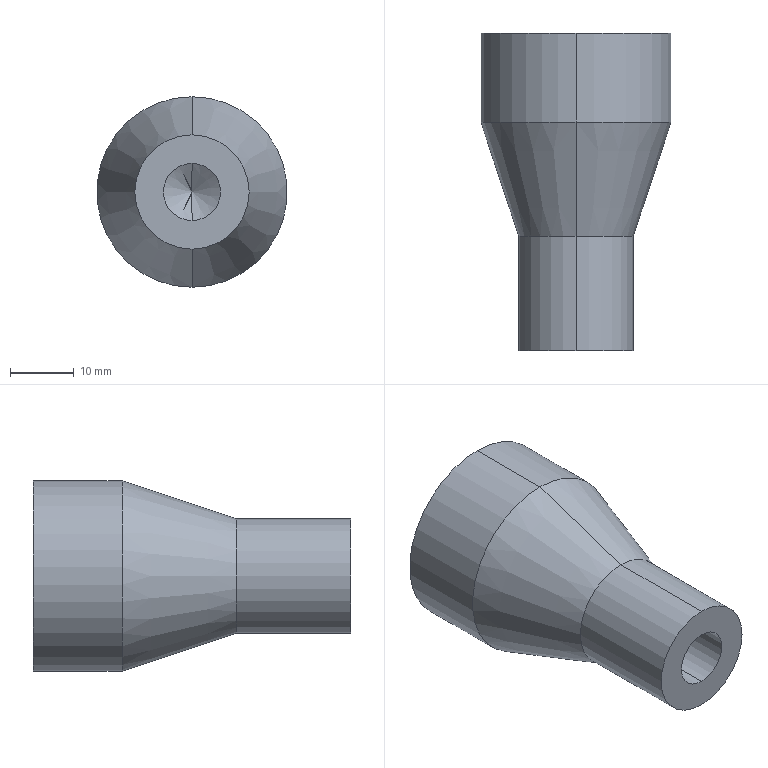Part | SolidWorks | features HoleWzd 2, Revolution 1 | 1 solid | 19 faces | box 30 x 50 x 30 mm | volume 17999 mm3 | cylinder 10 | cone 6 | plane 3 | commonest cylinder face diameters 3.3 x2 9 x2 18 x2 27 x2 30 x2
STEP:
#1=CARTESIAN_POINT('',(0.,34.9,-1.65));
#2=VERTEX_POINT('',#1);
#3=CARTESIAN_POINT('',(0.,34.9,1.65));
#4=VERTEX_POINT('',#3);
#5=CARTESIAN_POINT('',(0.,34.9,0.));
#6=DIRECTION('',(0.,1.,0.));
#7=DIRECTION('',(0.,0.,1.));
#8=AXIS2_PLACEMENT_3D('',#5,#6,#7);
#9=CIRCLE('',#8,1.65);
#10=EDGE_CURVE('',#2,#4,#9,.T.);
#11=ORIENTED_EDGE('',*,*,#10,.F.);
#12=CARTESIAN_POINT('',(0.,45.,-1.65));
#13=VERTEX_POINT('',#12);
#14=CARTESIAN_POINT('',(0.,45.,-1.65));
#15=DIRECTION('',(0.,1.,0.));
#16=VECTOR('',#15,1000.);
#17=LINE('',#14,#16);
#18=EDGE_CURVE('',#2,#13,#17,.T.);
#19=ORIENTED_EDGE('',*,*,#18,.T.);
#20=CARTESIAN_POINT('',(0.,45.,1.65));
#21=VERTEX_POINT('',#20);
#22=CARTESIAN_POINT('',(0.,45.,0.));
#23=DIRECTION('',(0.,1.,0.));
#24=DIRECTION('',(0.,0.,1.));
#25=AXIS2_PLACEMENT_3D('',#22,#23,#24);
#26=CIRCLE('',#25,1.65);
#27=EDGE_CURVE('',#13,#21,#26,.T.);
#28=ORIENTED_EDGE('',*,*,#27,.T.);
#29=CARTESIAN_POINT('',(0.,45.,1.65));
#30=DIRECTION('',(0.,1.,0.));
#31=VECTOR('',#30,1000.);
#32=LINE('',#29,#31);
#33=EDGE_CURVE('',#4,#21,#32,.T.);
#34=ORIENTED_EDGE('',*,*,#33,.F.);
#35=EDGE_LOOP('',(#11,#19,#28,#34));
#36=FACE_OUTER_BOUND('',#35,.T.);
#37=CARTESIAN_POINT('',(0.,45.,0.));
#38=DIRECTION('',(0.,1.,0.));
#39=DIRECTION('',(0.,0.,1.));
#40=AXIS2_PLACEMENT_3D('',#37,#38,#39);
#41=CYLINDRICAL_SURFACE('',#40,1.65);
#42=ADVANCED_FACE('',(#36),#41,.F.);
#43=CARTESIAN_POINT('',(0.,33.909,0.));
#44=VERTEX_POINT('',#43);
#45=CARTESIAN_POINT('',(0.,34.9,1.65));
#46=DIRECTION('',(0.,0.515,0.8572));
#47=VECTOR('',#46,1000.);
#48=LINE('',#45,#47);
#49=EDGE_CURVE('',#44,#4,#48,.T.);
#50=ORIENTED_EDGE('',*,*,#49,.F.);
#51=CARTESIAN_POINT('',(0.,34.9,-1.65));
#52=DIRECTION('',(0.,0.515,-0.8572));
#53=VECTOR('',#52,1000.);
#54=LINE('',#51,#53);
#55=EDGE_CURVE('',#44,#2,#54,.T.);
#56=ORIENTED_EDGE('',*,*,#55,.T.);
#57=ORIENTED_EDGE('',*,*,#10,.T.);
#58=EDGE_LOOP('',(#50,#56,#57));
#59=FACE_OUTER_BOUND('',#58,.T.);
#60=CARTESIAN_POINT('',(0.,34.9,0.));
#61=DIRECTION('',(0.,1.,0.));
#62=DIRECTION('',(0.,0.,1.));
#63=AXIS2_PLACEMENT_3D('',#60,#61,#62);
#64=CONICAL_SURFACE('',#63,1.65,1.03);
#65=ADVANCED_FACE('',(#59),#64,.F.);
#66=CARTESIAN_POINT('',(0.,28.,4.5));
#67=VERTEX_POINT('',#66);
#68=CARTESIAN_POINT('',(0.,28.,-4.5));
#69=VERTEX_POINT('',#68);
#70=CARTESIAN_POINT('',(0.,28.,0.));
#71=DIRECTION('',(0.,-1.,0.));
#72=DIRECTION('',(0.,0.,-1.));
#73=AXIS2_PLACEMENT_3D('',#70,#71,#72);
#74=CIRCLE('',#73,4.5);
#75=EDGE_CURVE('',#67,#69,#74,.T.);
#76=ORIENTED_EDGE('',*,*,#75,.F.);
#77=CARTESIAN_POINT('',(0.,0.,4.5));
#78=VERTEX_POINT('',#77);
#79=CARTESIAN_POINT('',(0.,0.,4.5));
#80=DIRECTION('',(0.,-1.,0.));
#81=VECTOR('',#80,1000.);
#82=LINE('',#79,#81);
#83=EDGE_CURVE('',#67,#78,#82,.T.);
#84=ORIENTED_EDGE('',*,*,#83,.T.);
#85=CARTESIAN_POINT('',(0.,0.,-4.5));
#86=VERTEX_POINT('',#85);
#87=CARTESIAN_POINT('',(0.,0.,0.));
#88=DIRECTION('',(0.,-1.,0.));
#89=DIRECTION('',(0.,0.,-1.));
#90=AXIS2_PLACEMENT_3D('',#87,#88,#89);
#91=CIRCLE('',#90,4.5);
#92=EDGE_CURVE('',#78,#86,#91,.T.);
#93=ORIENTED_EDGE('',*,*,#92,.T.);
#94=CARTESIAN_POINT('',(0.,0.,-4.5));
#95=DIRECTION('',(0.,-1.,0.));
#96=VECTOR('',#95,1000.);
#97=LINE('',#94,#96);
#98=EDGE_CURVE('',#69,#86,#97,.T.);
#99=ORIENTED_EDGE('',*,*,#98,.F.);
#100=EDGE_LOOP('',(#76,#84,#93,#99));
#101=FACE_OUTER_BOUND('',#100,.T.);
#102=CARTESIAN_POINT('',(0.,0.,0.));
#103=DIRECTION('',(0.,-1.,0.));
#104=DIRECTION('',(0.,0.,-1.));
#105=AXIS2_PLACEMENT_3D('',#102,#103,#104);
#106=CYLINDRICAL_SURFACE('',#105,4.5);
#107=ADVANCED_FACE('',(#101),#106,.F.);
#108=CARTESIAN_POINT('',(0.,30.704,0.));
#109=VERTEX_POINT('',#108);
#110=CARTESIAN_POINT('',(0.,28.,-4.5));
#111=DIRECTION('',(0.,-0.515,-0.8572));
#112=VECTOR('',#111,1000.);
#113=LINE('',#110,#112);
#114=EDGE_CURVE('',#109,#69,#113,.T.);
#115=ORIENTED_EDGE('',*,*,#114,.F.);
#116=CARTESIAN_POINT('',(0.,28.,4.5));
#117=DIRECTION('',(0.,-0.515,0.8572));
#118=VECTOR('',#117,1000.);
#119=LINE('',#116,#118);
#120=EDGE_CURVE('',#109,#67,#119,.T.);
#121=ORIENTED_EDGE('',*,*,#120,.T.);
#122=ORIENTED_EDGE('',*,*,#75,.T.);
#123=EDGE_LOOP('',(#115,#121,#122));
#124=FACE_OUTER_BOUND('',#123,.T.);
#125=CARTESIAN_POINT('',(0.,28.,0.));
#126=DIRECTION('',(0.,-1.,0.));
#127=DIRECTION('',(0.,0.,-1.));
#128=AXIS2_PLACEMENT_3D('',#125,#126,#127);
#129=CONICAL_SURFACE('',#128,4.5,1.03);
#130=ADVANCED_FACE('',(#124),#129,.F.);
#131=CARTESIAN_POINT('',(0.,45.,-13.5));
#132=VERTEX_POINT('',#131);
#133=CARTESIAN_POINT('',(0.,45.,13.5));
#134=VERTEX_POINT('',#133);
#135=CARTESIAN_POINT('',(0.,45.,0.));
#136=DIRECTION('',(0.,1.,0.));
#137=DIRECTION('',(0.,0.,1.));
#138=AXIS2_PLACEMENT_3D('',#135,#136,#137);
#139=CIRCLE('',#138,13.5);
#140=EDGE_CURVE('',#132,#134,#139,.T.);
#141=ORIENTED_EDGE('',*,*,#140,.F.);
#142=CARTESIAN_POINT('',(0.,50.,-13.5));
#143=VERTEX_POINT('',#142);
#144=CARTESIAN_POINT('',(0.,0.,-13.5));
#145=DIRECTION('',(0.,1.,0.));
#146=VECTOR('',#145,1000.);
#147=LINE('',#144,#146);
#148=EDGE_CURVE('',#132,#143,#147,.T.);
#149=ORIENTED_EDGE('',*,*,#148,.T.);
#150=CARTESIAN_POINT('',(0.,50.,13.5));
#151=VERTEX_POINT('',#150);
#152=CARTESIAN_POINT('',(0.,50.,0.));
#153=DIRECTION('',(0.,1.,0.));
#154=DIRECTION('',(0.,0.,1.));
#155=AXIS2_PLACEMENT_3D('',#152,#153,#154);
#156=CIRCLE('',#155,13.5);
#157=EDGE_CURVE('',#143,#151,#156,.T.);
#158=ORIENTED_EDGE('',*,*,#157,.T.);
#159=CARTESIAN_POINT('',(0.,0.,13.5));
#160=DIRECTION('',(0.,1.,0.));
#161=VECTOR('',#160,1000.);
#162=LINE('',#159,#161);
#163=EDGE_CURVE('',#134,#151,#162,.T.);
#164=ORIENTED_EDGE('',*,*,#163,.F.);
#165=EDGE_LOOP('',(#141,#149,#158,#164));
#166=FACE_OUTER_BOUND('',#165,.T.);
#167=CARTESIAN_POINT('',(0.,0.,0.));
#168=DIRECTION('',(0.,1.,0.));
#169=DIRECTION('',(0.,0.,1.));
#170=AXIS2_PLACEMENT_3D('',#167,#168,#169);
#171=CYLINDRICAL_SURFACE('',#170,13.5);
#172=ADVANCED_FACE('',(#166),#171,.F.);
#173=CARTESIAN_POINT('',(0.,36.,15.));
#174=VERTEX_POINT('',#173);
#175=CARTESIAN_POINT('',(0.,36.,-15.));
#176=VERTEX_POINT('',#175);
#177=CARTESIAN_POINT('',(0.,36.,0.));
#178=DIRECTION('',(0.,1.,0.));
#179=DIRECTION('',(0.,0.,1.));
#180=AXIS2_PLACEMENT_3D('',#177,#178,#179);
#181=CIRCLE('',#180,15.);
#182=EDGE_CURVE('',#174,#176,#181,.T.);
#183=ORIENTED_EDGE('',*,*,#182,.T.);
#184=CARTESIAN_POINT('',(0.,50.,-15.));
#185=VERTEX_POINT('',#184);
#186=CARTESIAN_POINT('',(0.,0.,-15.));
#187=DIRECTION('',(0.,1.,0.));
#188=VECTOR('',#187,1000.);
#189=LINE('',#186,#188);
#190=EDGE_CURVE('',#176,#185,#189,.T.);
#191=ORIENTED_EDGE('',*,*,#190,.T.);
#192=CARTESIAN_POINT('',(0.,50.,15.));
#193=VERTEX_POINT('',#192);
#194=CARTESIAN_POINT('',(0.,50.,0.));
#195=DIRECTION('',(0.,1.,0.));
#196=DIRECTION('',(0.,0.,1.));
#197=AXIS2_PLACEMENT_3D('',#194,#195,#196);
#198=CIRCLE('',#197,15.);
#199=EDGE_CURVE('',#193,#185,#198,.T.);
#200=ORIENTED_EDGE('',*,*,#199,.F.);
#201=CARTESIAN_POINT('',(0.,0.,15.));
#202=DIRECTION('',(0.,1.,0.));
#203=VECTOR('',#202,1000.);
#204=LINE('',#201,#203);
#205=EDGE_CURVE('',#174,#193,#204,.T.);
#206=ORIENTED_EDGE('',*,*,#205,.F.);
#207=EDGE_LOOP('',(#183,#191,#200,#206));
#208=FACE_OUTER_BOUND('',#207,.T.);
#209=CARTESIAN_POINT('',(0.,0.,0.));
#210=DIRECTION('',(0.,1.,0.));
#211=DIRECTION('',(0.,0.,1.));
#212=AXIS2_PLACEMENT_3D('',#209,#210,#211);
#213=CYLINDRICAL_SURFACE('',#212,15.);
#214=ADVANCED_FACE('',(#208),#213,.T.);
#215=CARTESIAN_POINT('',(0.,18.,9.));
#216=VERTEX_POINT('',#215);
#217=CARTESIAN_POINT('',(0.,18.,-9.));
#218=VERTEX_POINT('',#217);
#219=CARTESIAN_POINT('',(0.,18.,0.));
#220=DIRECTION('',(0.,1.,0.));
#221=DIRECTION('',(0.,0.,1.));
#222=AXIS2_PLACEMENT_3D('',#219,#220,#221);
#223=CIRCLE('',#222,9.);
#224=EDGE_CURVE('',#216,#218,#223,.T.);
#225=ORIENTED_EDGE('',*,*,#224,.T.);
#226=CARTESIAN_POINT('',(0.,36.,-15.));
#227=DIRECTION('',(0.,0.9487,-0.3162));
#228=VECTOR('',#227,1000.);
#229=LINE('',#226,#228);
#230=EDGE_CURVE('',#218,#176,#229,.T.);
#231=ORIENTED_EDGE('',*,*,#230,.T.);
#232=ORIENTED_EDGE('',*,*,#182,.F.);
#233=CARTESIAN_POINT('',(0.,36.,15.));
#234=DIRECTION('',(0.,0.9487,0.3162));
#235=VECTOR('',#234,1000.);
#236=LINE('',#233,#235);
#237=EDGE_CURVE('',#216,#174,#236,.T.);
#238=ORIENTED_EDGE('',*,*,#237,.F.);
#239=EDGE_LOOP('',(#225,#231,#232,#238));
#240=FACE_OUTER_BOUND('',#239,.T.);
#241=CARTESIAN_POINT('',(0.,36.,0.));
#242=DIRECTION('',(0.,1.,0.));
#243=DIRECTION('',(0.,0.,1.));
#244=AXIS2_PLACEMENT_3D('',#241,#242,#243);
#245=CONICAL_SURFACE('',#244,15.,0.3218);
#246=ADVANCED_FACE('',(#240),#245,.T.);
#247=CARTESIAN_POINT('',(0.,0.,9.));
#248=VERTEX_POINT('',#247);
#249=CARTESIAN_POINT('',(0.,0.,-9.));
#250=VERTEX_POINT('',#249);
#251=CARTESIAN_POINT('',(0.,0.,0.));
#252=DIRECTION('',(0.,1.,0.));
#253=DIRECTION('',(0.,0.,1.));
#254=AXIS2_PLACEMENT_3D('',#251,#252,#253);
#255=CIRCLE('',#254,9.);
#256=EDGE_CURVE('',#248,#250,#255,.T.);
#257=ORIENTED_EDGE('',*,*,#256,.T.);
#258=CARTESIAN_POINT('',(0.,0.,-9.));
#259=DIRECTION('',(0.,1.,0.));
#260=VECTOR('',#259,1000.);
#261=LINE('',#258,#260);
#262=EDGE_CURVE('',#250,#218,#261,.T.);
#263=ORIENTED_EDGE('',*,*,#262,.T.);
#264=ORIENTED_EDGE('',*,*,#224,.F.);
#265=CARTESIAN_POINT('',(0.,0.,9.));
#266=DIRECTION('',(0.,1.,0.));
#267=VECTOR('',#266,1000.);
#268=LINE('',#265,#267);
#269=EDGE_CURVE('',#248,#216,#268,.T.);
#270=ORIENTED_EDGE('',*,*,#269,.F.);
#271=EDGE_LOOP('',(#257,#263,#264,#270));
#272=FACE_OUTER_BOUND('',#271,.T.);
#273=CARTESIAN_POINT('',(0.,0.,0.));
#274=DIRECTION('',(0.,1.,0.));
#275=DIRECTION('',(0.,0.,1.));
#276=AXIS2_PLACEMENT_3D('',#273,#274,#275);
#277=CYLINDRICAL_SURFACE('',#276,9.);
#278=ADVANCED_FACE('',(#272),#277,.T.);
#279=CARTESIAN_POINT('',(0.,0.,0.));
#280=DIRECTION('',(0.,-1.,0.));
#281=DIRECTION('',(0.,0.,-1.));
#282=AXIS2_PLACEMENT_3D('',#279,#280,#281);
#283=CIRCLE('',#282,4.5);
#284=EDGE_CURVE('',#86,#78,#283,.T.);
#285=ORIENTED_EDGE('',*,*,#284,.F.);
#286=ORIENTED_EDGE('',*,*,#92,.F.);
#287=EDGE_LOOP('',(#285,#286));
#288=FACE_BOUND('',#287,.T.);
#289=ORIENTED_EDGE('',*,*,#256,.F.);
#290=CARTESIAN_POINT('',(0.,0.,0.));
#291=DIRECTION('',(0.,1.,0.));
#292=DIRECTION('',(0.,0.,1.));
#293=AXIS2_PLACEMENT_3D('',#290,#291,#292);
#294=CIRCLE('',#293,9.);
#295=EDGE_CURVE('',#250,#248,#294,.T.);
#296=ORIENTED_EDGE('',*,*,#295,.F.);
#297=EDGE_LOOP('',(#289,#296));
#298=FACE_OUTER_BOUND('',#297,.T.);
#299=CARTESIAN_POINT('',(0.,0.,0.));
#300=DIRECTION('',(0.,-1.,0.));
#301=DIRECTION('',(0.,0.,-1.));
#302=AXIS2_PLACEMENT_3D('',#299,#300,#301);
#303=PLANE('',#302);
#304=ADVANCED_FACE('',(#288,#298),#303,.T.);
#305=ORIENTED_EDGE('',*,*,#262,.F.);
#306=ORIENTED_EDGE('',*,*,#295,.T.);
#307=ORIENTED_EDGE('',*,*,#269,.T.);
#308=CARTESIAN_POINT('',(0.,18.,0.));
#309=DIRECTION('',(0.,1.,0.));
#310=DIRECTION('',(0.,0.,1.));
#311=AXIS2_PLACEMENT_3D('',#308,#309,#310);
#312=CIRCLE('',#311,9.);
#313=EDGE_CURVE('',#218,#216,#312,.T.);
#314=ORIENTED_EDGE('',*,*,#313,.F.);
#315=EDGE_LOOP('',(#305,#306,#307,#314));
#316=FACE_OUTER_BOUND('',#315,.T.);
#317=CARTESIAN_POINT('',(0.,0.,0.));
#318=DIRECTION('',(0.,1.,0.));
#319=DIRECTION('',(0.,0.,1.));
#320=AXIS2_PLACEMENT_3D('',#317,#318,#319);
#321=CYLINDRICAL_SURFACE('',#320,9.);
#322=ADVANCED_FACE('',(#316),#321,.T.);
#323=ORIENTED_EDGE('',*,*,#230,.F.);
#324=ORIENTED_EDGE('',*,*,#313,.T.);
#325=ORIENTED_EDGE('',*,*,#237,.T.);
#326=CARTESIAN_POINT('',(0.,36.,0.));
#327=DIRECTION('',(0.,1.,0.));
#328=DIRECTION('',(0.,0.,1.));
#329=AXIS2_PLACEMENT_3D('',#326,#327,#328);
#330=CIRCLE('',#329,15.);
#331=EDGE_CURVE('',#176,#174,#330,.T.);
#332=ORIENTED_EDGE('',*,*,#331,.F.);
#333=EDGE_LOOP('',(#323,#324,#325,#332));
#334=FACE_OUTER_BOUND('',#333,.T.);
#335=CARTESIAN_POINT('',(0.,36.,0.));
#336=DIRECTION('',(0.,1.,0.));
#337=DIRECTION('',(0.,0.,1.));
#338=AXIS2_PLACEMENT_3D('',#335,#336,#337);
#339=CONICAL_SURFACE('',#338,15.,0.3218);
#340=ADVANCED_FACE('',(#334),#339,.T.);
#341=ORIENTED_EDGE('',*,*,#190,.F.);
#342=ORIENTED_EDGE('',*,*,#331,.T.);
#343=ORIENTED_EDGE('',*,*,#205,.T.);
#344=CARTESIAN_POINT('',(0.,50.,0.));
#345=DIRECTION('',(0.,1.,0.));
#346=DIRECTION('',(0.,0.,1.));
#347=AXIS2_PLACEMENT_3D('',#344,#345,#346);
#348=CIRCLE('',#347,15.);
#349=EDGE_CURVE('',#185,#193,#348,.T.);
#350=ORIENTED_EDGE('',*,*,#349,.F.);
#351=EDGE_LOOP('',(#341,#342,#343,#350));
#352=FACE_OUTER_BOUND('',#351,.T.);
#353=CARTESIAN_POINT('',(0.,0.,0.));
#354=DIRECTION('',(0.,1.,0.));
#355=DIRECTION('',(0.,0.,1.));
#356=AXIS2_PLACEMENT_3D('',#353,#354,#355);
#357=CYLINDRICAL_SURFACE('',#356,15.);
#358=ADVANCED_FACE('',(#352),#357,.T.);
#359=ORIENTED_EDGE('',*,*,#199,.T.);
#360=ORIENTED_EDGE('',*,*,#349,.T.);
#361=EDGE_LOOP('',(#359,#360));
#362=FACE_OUTER_BOUND('',#361,.T.);
#363=CARTESIAN_POINT('',(0.,50.,0.));
#364=DIRECTION('',(0.,1.,0.));
#365=DIRECTION('',(0.,0.,1.));
#366=AXIS2_PLACEMENT_3D('',#363,#364,#365);
#367=CIRCLE('',#366,13.5);
#368=EDGE_CURVE('',#151,#143,#367,.T.);
#369=ORIENTED_EDGE('',*,*,#368,.F.);
#370=ORIENTED_EDGE('',*,*,#157,.F.);
#371=EDGE_LOOP('',(#369,#370));
#372=FACE_BOUND('',#371,.T.);
#373=CARTESIAN_POINT('',(-15.,50.,0.));
#374=DIRECTION('',(0.,1.,0.));
#375=DIRECTION('',(0.,0.,1.));
#376=AXIS2_PLACEMENT_3D('',#373,#374,#375);
#377=PLANE('',#376);
#378=ADVANCED_FACE('',(#362,#372),#377,.T.);
#379=ORIENTED_EDGE('',*,*,#148,.F.);
#380=CARTESIAN_POINT('',(0.,45.,0.));
#381=DIRECTION('',(0.,1.,0.));
#382=DIRECTION('',(0.,0.,1.));
#383=AXIS2_PLACEMENT_3D('',#380,#381,#382);
#384=CIRCLE('',#383,13.5);
#385=EDGE_CURVE('',#134,#132,#384,.T.);
#386=ORIENTED_EDGE('',*,*,#385,.F.);
#387=ORIENTED_EDGE('',*,*,#163,.T.);
#388=ORIENTED_EDGE('',*,*,#368,.T.);
#389=EDGE_LOOP('',(#379,#386,#387,#388));
#390=FACE_OUTER_BOUND('',#389,.T.);
#391=CARTESIAN_POINT('',(0.,0.,0.));
#392=DIRECTION('',(0.,1.,0.));
#393=DIRECTION('',(0.,0.,1.));
#394=AXIS2_PLACEMENT_3D('',#391,#392,#393);
#395=CYLINDRICAL_SURFACE('',#394,13.5);
#396=ADVANCED_FACE('',(#390),#395,.F.);
#397=CARTESIAN_POINT('',(0.,45.,0.));
#398=DIRECTION('',(0.,1.,0.));
#399=DIRECTION('',(0.,0.,1.));
#400=AXIS2_PLACEMENT_3D('',#397,#398,#399);
#401=CIRCLE('',#400,1.65);
#402=EDGE_CURVE('',#21,#13,#401,.T.);
#403=ORIENTED_EDGE('',*,*,#402,.F.);
#404=ORIENTED_EDGE('',*,*,#27,.F.);
#405=EDGE_LOOP('',(#403,#404));
#406=FACE_BOUND('',#405,.T.);
#407=ORIENTED_EDGE('',*,*,#385,.T.);
#408=ORIENTED_EDGE('',*,*,#140,.T.);
#409=EDGE_LOOP('',(#407,#408));
#410=FACE_OUTER_BOUND('',#409,.T.);
#411=CARTESIAN_POINT('',(-13.5,45.,0.));
#412=DIRECTION('',(0.,1.,0.));
#413=DIRECTION('',(0.,0.,1.));
#414=AXIS2_PLACEMENT_3D('',#411,#412,#413);
#415=PLANE('',#414);
#416=ADVANCED_FACE('',(#406,#410),#415,.T.);
#417=ORIENTED_EDGE('',*,*,#120,.F.);
#418=ORIENTED_EDGE('',*,*,#114,.T.);
#419=CARTESIAN_POINT('',(0.,28.,0.));
#420=DIRECTION('',(0.,-1.,0.));
#421=DIRECTION('',(0.,0.,-1.));
#422=AXIS2_PLACEMENT_3D('',#419,#420,#421);
#423=CIRCLE('',#422,4.5);
#424=EDGE_CURVE('',#69,#67,#423,.T.);
#425=ORIENTED_EDGE('',*,*,#424,.T.);
#426=EDGE_LOOP('',(#417,#418,#425));
#427=FACE_OUTER_BOUND('',#426,.T.);
#428=CARTESIAN_POINT('',(0.,28.,0.));
#429=DIRECTION('',(0.,-1.,0.));
#430=DIRECTION('',(0.,0.,-1.));
#431=AXIS2_PLACEMENT_3D('',#428,#429,#430);
#432=CONICAL_SURFACE('',#431,4.5,1.03);
#433=ADVANCED_FACE('',(#427),#432,.F.);
#434=ORIENTED_EDGE('',*,*,#83,.F.);
#435=ORIENTED_EDGE('',*,*,#424,.F.);
#436=ORIENTED_EDGE('',*,*,#98,.T.);
#437=ORIENTED_EDGE('',*,*,#284,.T.);
#438=EDGE_LOOP('',(#434,#435,#436,#437));
#439=FACE_OUTER_BOUND('',#438,.T.);
#440=CARTESIAN_POINT('',(0.,0.,0.));
#441=DIRECTION('',(0.,-1.,0.));
#442=DIRECTION('',(0.,0.,-1.));
#443=AXIS2_PLACEMENT_3D('',#440,#441,#442);
#444=CYLINDRICAL_SURFACE('',#443,4.5);
#445=ADVANCED_FACE('',(#439),#444,.F.);
#446=ORIENTED_EDGE('',*,*,#55,.F.);
#447=ORIENTED_EDGE('',*,*,#49,.T.);
#448=CARTESIAN_POINT('',(0.,34.9,0.));
#449=DIRECTION('',(0.,1.,0.));
#450=DIRECTION('',(0.,0.,1.));
#451=AXIS2_PLACEMENT_3D('',#448,#449,#450);
#452=CIRCLE('',#451,1.65);
#453=EDGE_CURVE('',#4,#2,#452,.T.);
#454=ORIENTED_EDGE('',*,*,#453,.T.);
#455=EDGE_LOOP('',(#446,#447,#454));
#456=FACE_OUTER_BOUND('',#455,.T.);
#457=CARTESIAN_POINT('',(0.,34.9,0.));
#458=DIRECTION('',(0.,1.,0.));
#459=DIRECTION('',(0.,0.,1.));
#460=AXIS2_PLACEMENT_3D('',#457,#458,#459);
#461=CONICAL_SURFACE('',#460,1.65,1.03);
#462=ADVANCED_FACE('',(#456),#461,.F.);
#463=ORIENTED_EDGE('',*,*,#18,.F.);
#464=ORIENTED_EDGE('',*,*,#453,.F.);
#465=ORIENTED_EDGE('',*,*,#33,.T.);
#466=ORIENTED_EDGE('',*,*,#402,.T.);
#467=EDGE_LOOP('',(#463,#464,#465,#466));
#468=FACE_OUTER_BOUND('',#467,.T.);
#469=CARTESIAN_POINT('',(0.,45.,0.));
#470=DIRECTION('',(0.,1.,0.));
#471=DIRECTION('',(0.,0.,1.));
#472=AXIS2_PLACEMENT_3D('',#469,#470,#471);
#473=CYLINDRICAL_SURFACE('',#472,1.65);
#474=ADVANCED_FACE('',(#468),#473,.F.);
#475=CLOSED_SHELL('',(#42,#65,#107,#130,#172,#214,#246,#278,#304,#322,#340,#358,#378,#396,#416,#433,#445,#462,#474));
#476=MANIFOLD_SOLID_BREP('',#475);
#477=CARTESIAN_POINT('',(0.,0.,0.));
#478=DIRECTION('',(0.,0.,1.));
#479=DIRECTION('',(1.,0.,0.));
#480=AXIS2_PLACEMENT_3D('',#477,#478,#479);
#481=(LENGTH_UNIT()NAMED_UNIT(*)SI_UNIT(.MILLI.,.METRE.));
#482=UNCERTAINTY_MEASURE_WITH_UNIT(LENGTH_MEASURE(0.00001),#481,'','');
#483=(NAMED_UNIT(*)PLANE_ANGLE_UNIT()SI_UNIT($,.RADIAN.));
#484=(NAMED_UNIT(*)SI_UNIT($,.STERADIAN.)SOLID_ANGLE_UNIT());
#485=(GEOMETRIC_REPRESENTATION_CONTEXT(3)GLOBAL_UNCERTAINTY_ASSIGNED_CONTEXT((#482))GLOBAL_UNIT_ASSIGNED_CONTEXT((#481,#483,#484))REPRESENTATION_CONTEXT('',''));
#486=ADVANCED_BREP_SHAPE_REPRESENTATION('',(#476,#480),#485);